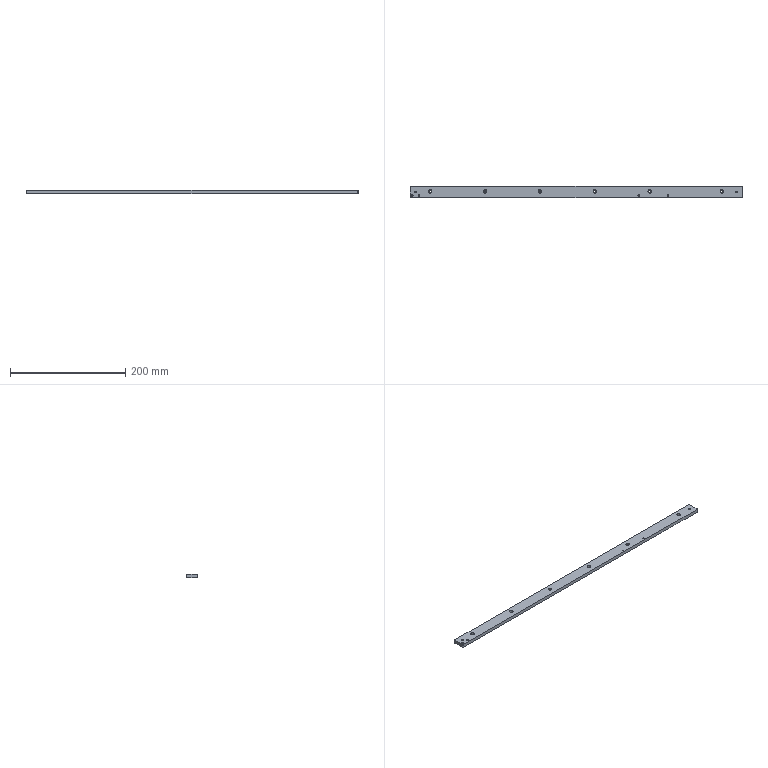Part | SolidWorks | features BaseBody 1 | 1 solid | 64 faces | box 575 x 20 x 6 mm | volume 67891 mm3 | cylinder 42 | plane 16 | cone 6 | commonest cylinder face diameters 2.459 x14 3.5 x12 6 x12 3.242 x4